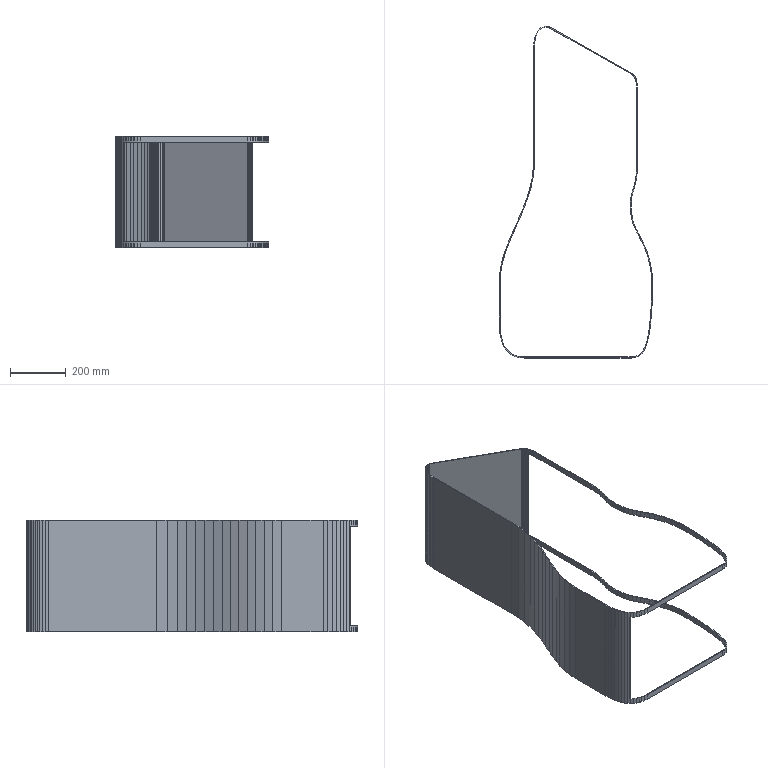Part | SolidWorks | features ICE 2, Extrusion 1 | 1 solid | 358 faces | box 552.5 x 1195 x 400 mm | volume 2091406 mm3 | plane 358